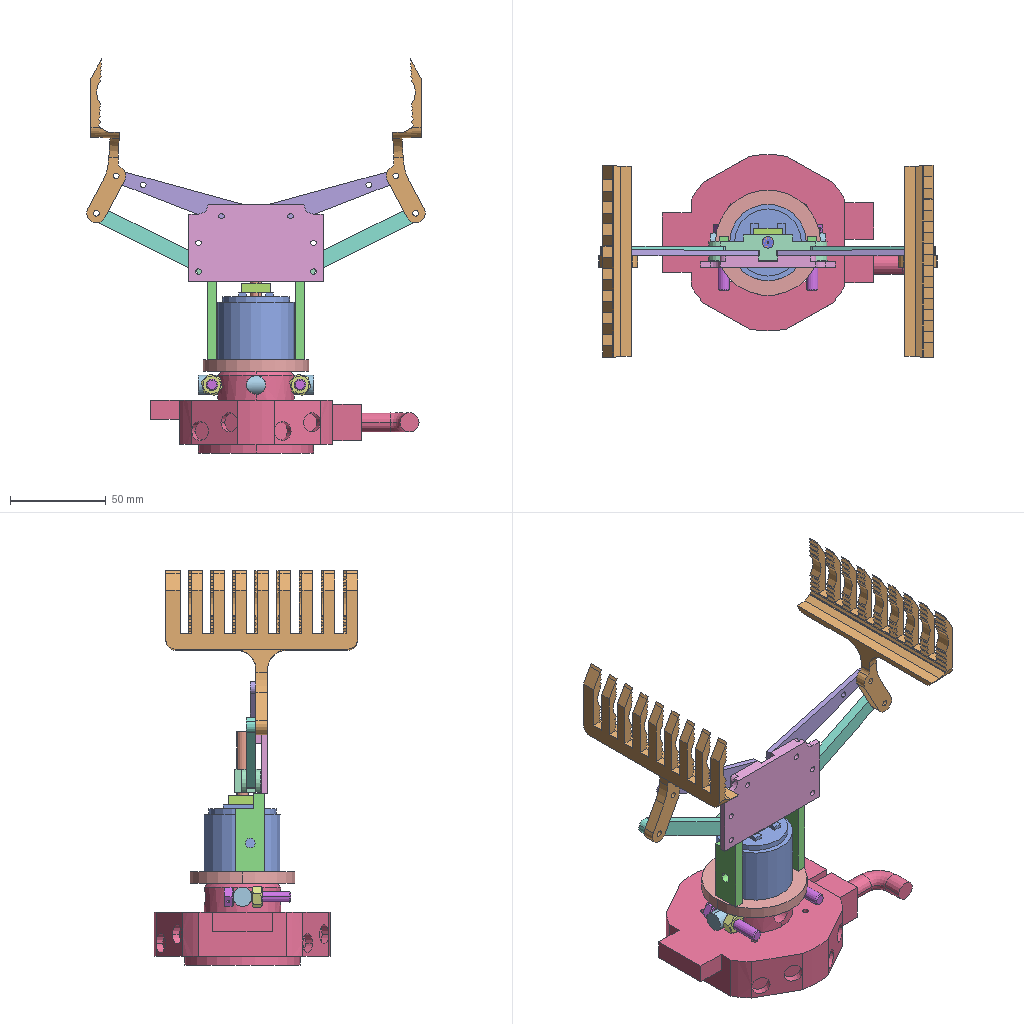Assembly | SolidWorks | 14 different items | 18 placed | box 176 x 106 x 206 mm
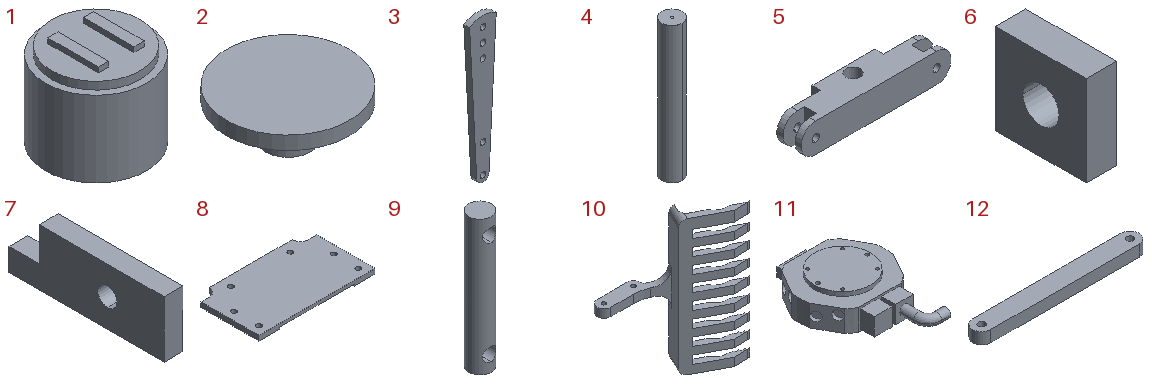Parts list (item | name | quantity | size | volume | features):
1 | - | x1 | 40 x 40 x 35 mm | 40905 mm3 | features MBimport 1
2 | - | x1 | 55 x 55 x 21 mm | 16595 mm3 | features ICE 2, CirPattern 1, MBimport 1
3 | - | x2 | 13.735 x 3 x 74.656 mm | 2101 mm3 | features ICE 3, BaseBody 1
4 | - | x1 | - | - | features MBimport 1
5 | - | x1 | 62 x 13.5 x 12 mm | 6888 mm3 | features ICE 4, Extrusion 1, MirrorSolid 1
6 | - | x1 | 5 x 15 x 15 mm | 983.628 mm3 | features MBimport 1
7 | - | x2 | 5 x 41 x 15 mm | 2617 mm3 | features ICE 2, MBimport 1
8 | - | x1 | 70 x 40 x 6 mm | 8316 mm3 | features ICE 2, MBimport 1
9 | - | x1 | 10 x 10 x 60 mm | 4174 mm3 | features Extrusion 1, ICE 1
10 | - | x2 | 77.412 x 40.573 x 100 mm | 15477 mm3 | features ICE 7, Fillet 2, Extrusion 1
11 | - | x1 | 92 x 140 x 42.6 mm | 179973 mm3 | features ICE 1, MBimport 1
12 | - | x2 | 73 x 8 x 5 mm | 2781 mm3 | features Extrusion 1, ICE 1
13 | hex bolts with wire hole-grade ab gb.sldQBX | x1 | - | - | -
14 | hex nuts, style 1-grades ab gb.sldQBX | x1 | - | - | -
Mates (type | each side: item.copy, entity, surface, feature):
Concentric | 2.1 face cylinder MotorBase.QBX.1<1> | 1.1 face cylinder Motor.QBX.1<1>
Coincident | 2.1 face plane MotorBase.QBX.1<1> | 1.1 face plane Motor.QBX.1<1>
Coincident | 1.1 face plane Motor.QBX.1<1> | 6.1 face plane SidePlate.QBX.1<1>
DistanceDim | 6.1 face plane SidePlate.QBX.1<1> | 1.1 face plane Motor.QBX.1<1> | 2 times
Concentric | 6.1 face cylinder SidePlate.QBX.1<1> | 4.1 face cylinder LeadScrew.QBX.1<1>
Coincident | 1.1 face plane Motor.QBX.1<1> | 4.1 face plane LeadScrew.QBX.1<1>
Concentric | 4.1 face cylinder LeadScrew.QBX.1<1> | assembly face
Concentric | assembly face | assembly face
Coincident | assembly face | assembly face
Parallel | 6.1 face plane SidePlate.QBX.1<1> | 8.1 face plane RearPlate.QBX.1<1>
DistanceDim | assembly face | 8.1 face plane RearPlate.QBX.1<1>
DistanceDim | 8.1 face plane RearPlate.QBX.1<1> | 6.1 face plane SidePlate.QBX.1<1>
Coincident | assembly face | 12.1 face plane Boss-Extrude1
Concentric | assembly face | 12.1 edge
Concentric | 12.2 edge | 10.1 face cylinder Boss-Extrude1
Coincident | 12.2 face plane Boss-Extrude1 | 10.1 face plane Boss-Extrude1
Coincident | 10.1 face plane Boss-Extrude1 | 3.1 face plane Input1
Concentric | 8.1 edge | 3.1 face cylinder Input1
Parallel | assembly face | assembly face
Concentric | 10.1 face cylinder Boss-Extrude1 | 3.1 face cylinder Boss-Extrude3
Parallel | 8.1 face plane RearPlate.QBX.1<1> | 10.1 face plane Boss-Extrude2
LimitDistanceDim | 4.1 face plane LeadScrew.QBX.1<1> | assembly face
Parallel | 8.1 face plane RearPlate.QBX.1<1> | 7.1 face plane SideUprightPlate.QBX.1<1>
Coincident | 2.1 face plane MotorBase.QBX.1<1> | 7.1 face plane SideUprightPlate.QBX.1<1>
Coincident | 8.1 face plane RearPlate.QBX.1<1> | 7.1 face plane Boss-Extrude1
DistanceDim | 7.1 face plane SideUprightPlate.QBX.1<1> | 8.1 face plane RearPlate.QBX.1<1>
Concentric | 2.1 face cylinder Boss-Extrude1 | 11.1 face cylinder Cut-Extrude1
Parallel | 2.1 face surface:4009 Cut-Extrude1 | 11.1 face cylinder Part 16.stp<1>
Coincident | 2.1 face plane MotorBase.QBX.1<1> | 11.1 face plane Part 16.stp<1>
Concentric | 11.1 face cylinder Part 16.stp<1> | 9.1 face cylinder Boss-Extrude1
Parallel | 11.1 face cylinder Part 16.stp<1> | 9.1 face cylinder Cut-Extrude1
DistanceDim | 9.1 face cylinder Cut-Extrude1 | 11.1 face cylinder Part 16.stp<1>
Parallel | 9.1 face plane Boss-Extrude1 | assembly face
DistanceDim | assembly face | 2.1 face plane MotorBase.QBX.1<1>
DistanceDim | assembly face | 9.1 face plane Boss-Extrude1
DistanceDim | assembly edge | assembly plane
Concentric | 4.1 face cylinder LeadScrew.QBX.1<1> | 5.1 face cylinder Cut-Extrude2
Parallel | 8.1 face plane RearPlate.QBX.1<1> | assembly plane
Parallel | 8.1 face plane RearPlate.QBX.1<1> | 5.1 face plane Boss-Extrude6
Concentric | 12.2 face cylinder Cut-Extrude1 | 5.1 face cylinder Mirror1
LimitDistanceDim | 6.1 face plane SidePlate.QBX.1<1> | 5.1 face plane Boss-Extrude1